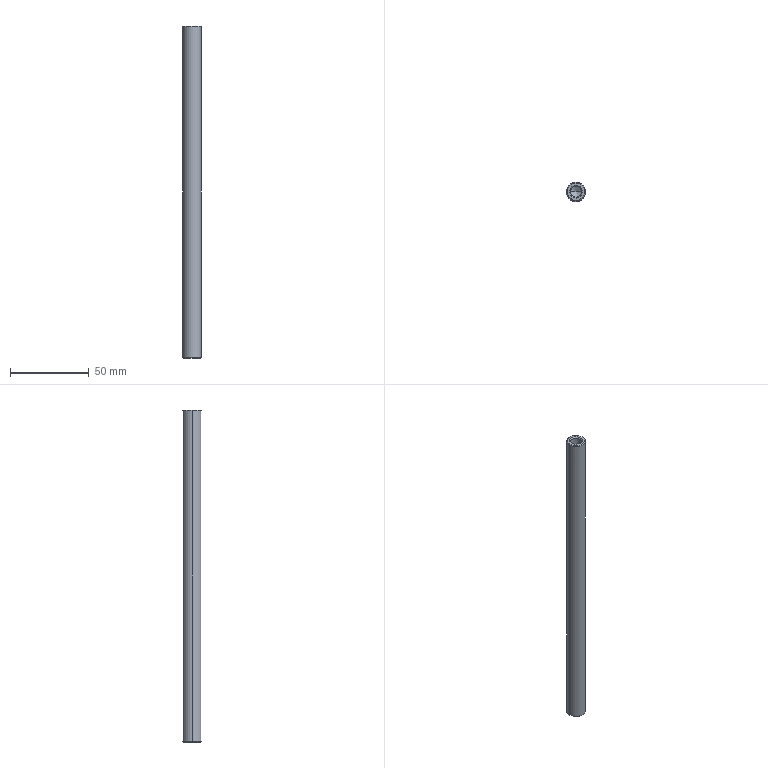Part | STEP file | 12C_A-1 | 1 solid | 20 faces | box 12 x 12 x 211 mm | volume 22253 mm3 | cone 12 | cylinder 6 | plane 2 | commonest cylinder face diameters 6.8 x4 12 x2